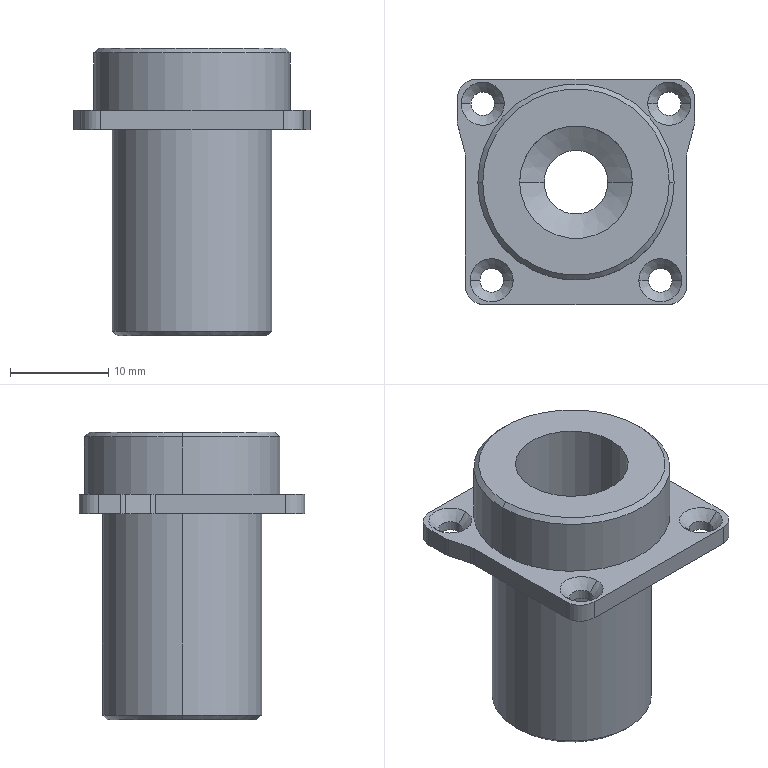NC program | NX | posted with a generic post | part box 24.2 x 23 x 29.342 mm
Whole program:
N10 G17 G21 G94 G90
(PLANAR_MILL , TOOL : D50面刀)
N12 T01 M6
N14 G53
N16 G17 G0 G90 X-0.5 Y-40.1 S4500 M3
N18 G43 Z20. H1
N20 Z2.
N22 G94 G1 Z0. F600.
N24 Y-12.1
N26 Y12.1
N28 Y40.1
N30 Z2.
N32 G0 Z20.
N34 M5
(动态粗 , TOOL : D8-25-D8-60-3T-ROUGH)
N36 T02 M6
N38 G53
N40 G17 G0 G90 X0.429 Y20.061 S6500 M3
N42 G43 Z20. H2
N44 Z-20.35
N46 G94 G1 X0.43 Y20.036 Z-20.506 F3000.
N48 X0.431 Y20.011 Z-20.568
N50 X0.432 Y19.986 Z-20.613
N52 X0.434 Y19.961 Z-20.65
N54 X0.435 Y19.936 Z-20.681
N56 X0.436 Y19.911 Z-20.707
N58 X0.437 Y19.886 Z-20.73
N60 X0.438 Y19.861 Z-20.75
N62 X0.44 Y19.836 Z-20.768
N64 X0.441 Y19.811 Z-20.783
N66 X0.442 Y19.786 Z-20.797
N68 X0.443 Y19.761 Z-20.808
N70 X0.444 Y19.736 Z-20.818
N72 X0.446 Y19.711 Z-20.827
N74 X0.447 Y19.686 Z-20.834
N76 X0.448 Y19.661 Z-20.84
N78 X0.449 Y19.636 Z-20.844
N80 X0.45 Y19.611 Z-20.847
N82 X0.452 Y19.586 Z-20.849
N84 X0.453 Y19.561 Z-20.85
N86 X0.516 Y18.254
N88 G3 X0.99 Y17.557 R0.809
N90 X3.846 Y16.911 R8.421
N92 X10.454 Y16.699 R95.671
N94 G2 X13.454 Y14.982 R4.502
N96 X15.139 Y11.177 R8.706
N98 X15.634 Y5.867 R30.68
N100 X15.682 Y-11.513 R786.797
N102 X13.805 Y-14.605 R4.562
N104 X9.896 Y-16.198 R9.151
N106 X4.22 Y-16.649 R35.622
N108 X-10.491 Y-16.683 R805.734
N110 X-13.56 Y-14.878 R4.516
N112 X-15.165 Y-11.103 R8.828
N114 X-15.645 Y-5.49 R33.344
N116 X-15.684 Y11.491 R889.228
N118 X-13.878 Y14.559 R4.516
N120 X-10.162 Y16.152 R8.771
N122 X-4.791 Y16.637 R31.617
N124 X-0.773 Y16.63 R41.473
N126 G3 X4.691 Y16.093 R140.668
N128 G2 X8.411 Y15.922 R235.686
N130 X12.726 Y13.128 R6.126
N132 X14.387 Y8.598 R11.548
N134 X14.854 Y2.08 R44.461
N136 X14.885 Y-9.139 R699.319
N138 X12.271 Y-13.604 R5.956
N140 X7.888 Y-15.33 R10.972
N142 X1.736 Y-15.839 R38.769
N144 X-8.283 Y-15.875 R261.049
N146 X-12.684 Y-13.17 R5.998
N148 X-14.357 Y-8.763 R11.22
N150 X-14.846 Y-2.489 R40.851
N152 X-14.877 Y9.271 R378.584
N154 X-12.178 Y13.678 R5.986
N156 X-7.775 Y15.354 R11.211
N158 X0.715 Y15.603 R31.798
N160 G3 X6.56 Y15.199 R403.425
N162 G2 X11.957 Y11.622 R7.16
N164 X13.598 Y6.695 R13.544
N166 X14.047 Y-0.005 R50.406
N168 X14.067 Y-7.426 R173.713
N170 X10.784 Y-12.81 R6.926
N172 X5.96 Y-14.546 R12.736
N174 X-0.496 Y-15.039 R44.911
N176 X-6.435 Y-15.064 R119.403
N178 X-11.831 Y-11.759 R6.914
N180 X-13.555 Y-6.914 R12.852
N182 X-14.048 Y-0.098 R47.277
N184 X-14.066 Y7.461 R161.04
N186 X-10.706 Y12.864 R6.932
N188 X-5.751 Y14.58 R12.98
N190 X0.415 Y14.758 R29.731
N192 X5.144 Y14.453 R98.986
N194 X11.196 Y10.249 R7.942
N196 X12.796 Y5.122 R15.097
N198 X13.082 Y2.379 R49.141
N200 G1 X13.293 Y0.888
N202 G2 X13.259 Y-5.834 R187.6
N204 X9.361 Y-12.067 R7.65
N206 X4.26 Y-13.762 R14.309
N208 X-2.558 Y-14.242 R51.282
N210 X-5.85 Y-14.118 R16.984
N212 X-11.092 Y-10.317 R7.64
N214 X-12.771 Y-5.208 R14.441
N216 X-13.25 Y1.911 R53.484
N218 X-13.225 Y6.169 R46.387
N220 X-9.465 Y12.006 R7.59
N222 X-3.951 Y13.739 R13.317
N224 X4.014 Y13.658 R40.114
N226 X10.324 Y9.169 R8.456
N228 X11.402 Y6.559 R14.95
N230 G1 X11.928 Y5.7
N232 X12.601 Y4.163
N234 G2 X13.084 Y2.371 R18.917
N236 G1 X13.293 Y0.888
N238 X13.3 Y-0.789
N240 X13.079 Y-2.452
N242 G3 X12.63 Y-4.819 R16.341
N244 G2 X7.704 Y-11.516 R8.73
N246 X2.295 Y-13.038 R16.937
N248 X-3.689 Y-13.355 R35.26
N250 X-10.12 Y-9.354 R8.001
N252 X-11.891 Y-4.223 R14.57
N254 X-12.436 Y3.19 R50.486
N256 X-11.797 Y7.249 R9.919
N258 X-7.419 Y11.614 R8.469
N260 X-1.95 Y12.889 R15.636
N262 X3.019 Y12.805 R23.293
N264 X8.22 Y9.955 R8.579
N266 G1 X8.764 Y9.572
N268 X9.992 Y8.429
N270 X11.053 Y7.131
N272 X11.428 Y6.516
N274 X11.053 Y7.131
N276 X9.992 Y8.429
N278 X8.764 Y9.572
N280 X7.392 Y10.538
N282 G3 X5.512 Y11.463 R17.868
N284 X0.467 Y12.382 R14.195
N286 X-5.693 Y11.598 R18.155
N288 X-10.208 Y8.351 R8.688
N290 X-11.688 Y3.96 R9.487
N292 X-11.08 Y-5.339 R29.025
N294 X-8.797 Y-9.934 R10.858
N296 X-3.703 Y-12.54 R8.228
N298 X5.606 Y-11.71 R21.642
N300 X10.229 Y-8.511 R9.469
N302 X11.104 Y-7.056 R10.021
N304 G1 X11.964 Y-5.629
N306 X12.63 Y-4.079
N308 X12.949 Y-2.922
N310 X12.63 Y-4.079
N312 X11.964 Y-5.629
N314 X11.093 Y-7.074
N316 X10.032 Y-8.386
N318 X8.801 Y-9.542
N320 X7.425 Y-10.518
N322 X5.928 Y-11.297
N324 X4.339 Y-11.864
N326 X2.687 Y-12.209
N328 X1.003 Y-12.325
N330 G2 X-2.002 Y-11.954 R14.341
N332 X-6.309 Y-10.392 R9.852
N334 X-9.345 Y-6.682 R9.353
N336 X-10.208 Y-5.126 R17.403
N338 G1 X-10.784 Y-3.612
N340 X-11.156 Y-2.035
N342 X-11.318 Y-0.423
N344 X-11.267 Y1.197
N346 G2 X-10.661 Y4.561 R41.802
N348 X-6.023 Y10.097 R8.435
N350 G1 X-5.47 Y10.49
N352 X-3.962 Y11.282
N354 X-2.36 Y11.858
N356 X-0.693 Y12.208
N358 X1.004 Y12.325
N360 X2.679 Y12.21
N362 X1.004 Y12.325
N364 X-0.693 Y12.208
N366 X-2.36 Y11.858
N368 X-3.962 Y11.282
N370 X-5.47 Y10.49
N372 X-6.79 Y9.551
N374 X-7.976 Y8.446
N376 X-9.006 Y7.196
N378 X-9.864 Y5.821
N380 X-10.533 Y4.346
N382 X-11.004 Y2.796
N384 X-11.267 Y1.197
N386 X-11.318 Y-0.423
N388 X-11.156 Y-2.035
N390 X-10.784 Y-3.612
N392 X-10.208 Y-5.126
N394 G3 X-9.345 Y-6.682 R17.403
N396 G1 X-8.489 Y-7.865
N398 X-7.376 Y-9.042
N400 X-6.117 Y-10.062
N402 G3 X-2.002 Y-11.954 R13.361
N404 G2 X-1.458 Y-12.57 R0.802
N406 G1 X-1.14 Y-14.109 Z-20.75
N408 X-1.099 Y-14.308 F15000.
N410 X-1.048 Y-14.504
N412 G3 X-0.234 Y-15.016 R0.8
N414 G1 X0.903 Y-14.921
N416 X2.038 Y-14.79
N418 G3 X4.321 Y-14.371 R24.733
N420 X6.908 Y-13.481 R14.428
N422 X8.603 Y-12.513 R11.909
N424 G1 X10.346 Y-11.305
N426 G3 X11.628 Y-10.293 R18.424
N428 X12.658 Y-9.047 R5.858
N430 X14.327 Y-6.159 R39.578
N432 X15.172 Y-4.349 R23.342
N434 X15.743 Y-0.988 R8.479
N436 G1 X15.709 Y0.018
N438 X15.664 Y1.025
N440 G3 X14.752 Y5.24 R15.147
N442 G1 X14.258 Y6.543
N444 G3 X12.967 Y8.697 R9.153
N446 X10.921 Y10.825 R16.919
N448 G1 X9.318 Y12.223
N450 G3 X8.424 Y12.331 R0.801
N452 G1 X8.332 Y12.283
N454 X6.937 Y11.559 Z-20.85 F3000.
N456 X6.681 Y11.423
N458 X6.417 Y11.301
N460 G2 X5.902 Y11.308 R0.808
N462 G1 X4.321 Y11.869
N464 X2.853 Y12.174
N466 G2 X2.212 Y12.895 R0.808
N468 G1 X2.097 Y14.219
N470 X2.095 Y14.244 Z-20.849
N472 X2.093 Y14.269 Z-20.847
N474 X2.091 Y14.294 Z-20.844
N476 X2.089 Y14.319 Z-20.84
N478 X2.086 Y14.344 Z-20.834
N480 X2.084 Y14.369 Z-20.827
N482 X2.082 Y14.394 Z-20.818
N484 X2.08 Y14.419 Z-20.808
N486 X2.078 Y14.443 Z-20.797
N488 X2.076 Y14.468 Z-20.783
N490 X2.073 Y14.493 Z-20.768
N492 X2.071 Y14.518 Z-20.75
N494 X2.069 Y14.543 Z-20.73
N496 X2.067 Y14.568 Z-20.707
N498 X2.065 Y14.593 Z-20.681
N500 X2.063 Y14.618 Z-20.65
N502 X2.06 Y14.643 Z-20.613
N504 X2.058 Y14.668 Z-20.568
N506 X2.056 Y14.692 Z-20.506
N508 X2.054 Y14.717 Z-20.35
N510 G0 Z20.
N512 M5
(DRILLING , TOOL : 倒角D4-90度)
N514 T05 M6
N516 G53
N518 G17 G0 G90 X1. Y0. S2000 M3
N520 G43 Z20. H5
N522 G94 G81 G99 Z-1. F200. R3.
N524 G80
N526 G0 X1. Y0. Z20.
N528 M5
(DRILLING_COPY , TOOL : 钻头D6.5-73-105)
N530 T06 M6
N532 G53
N534 G17 G0 G90 X1. Y0. S2000 M3
N536 G43 Z20. H6
N538 G94 G83 G99 Z-32. F200. Q2. R3.
N540 G80
N542 G0 X1. Y0. Z20.
N544 M5
(动态粗_1 , TOOL : D4-12-D4-50-3T-ROUGH)
N546 T04 M6
N548 G53
N550 G17 G0 G90 X1. Y0. S5500 M3
N552 G43 Z20. H4
N554 Z-9.25
N556 G94 G1 Z-9.75 F1500.
N558 G3 X0.983 Y-0.392 R0.198
N560 X1.196 Y0.415 R0.42
N562 X1.105 Y-0.473 R-0.467
N564 X0.551 Y0.282 R-0.514
N566 X1.453 Y0.402 R-0.565
N568 X1.019 Y-0.64 R-0.618
N570 X0.554 Y0.544 R-0.677
N572 X1.783 Y0.083 R-0.74
N574 X0.511 Y-0.666 R-0.806
N576 X1.06 Y0.919 R-0.877
N578 X1.529 Y-0.837 R-0.95
N580 X-0.003 Y0.334 R-1.028
N582 X2.106 Y0.383 R-1.111
N584 X0.222 Y-0.946 R-1.197
N586 X1.375 Y1.287 R-1.285
N588 X1.252 Y-1.395 R-1.376
N590 X0.226 Y1.305 R-1.47
N592 X2.331 Y-0.933 R-1.568
N594 X-0.651 Y0.439 R-1.669
N596 X2.829 Y0.208 R-1.773
N598 X-0.732 Y-0.822 R-1.88
N600 X2.557 Y1.349 R-1.989
N602 X-0.217 Y-1.762 R-2.1
N604 X1.893 Y2.1 R-2.212
N606 X0.518 Y-2.325 R-2.327
N608 X1.127 Y2.508 R-2.444
N610 X1.307 Y-2.6 R-2.563
N612 X0.246 Y2.644 R-2.685
N614 X2.252 Y-2.583 R-2.809
N616 X-0.664 Y2.491 R-2.934
N618 X3.08 Y-2.338 R-3.062
N620 X-1.336 Y2.257 R-3.19
N622 X3.611 Y-2.163 R-3.319
N624 X-1.599 Y2.352 R3.447
N626 X3.801 Y-2.339 R-3.577
N628 X-1.848 Y2.467 R3.708
N630 X4.026 Y-2.485 R-3.841
N632 X3.583 Y3.015 R3.941
N634 X0.212 Y3.891 R4.103
N636 X-2.093 Y2.488 R4.209
N638 X-2.969 Y-0.064 R4.209
N640 X-2.018 Y-2.579 R4.208
N642 X0.318 Y-3.911 R4.208
N644 X2.965 Y-3.45 R4.203
N646 X4.585 Y1.699 R4.003
N648 X3.606 Y2.995 R4.316
N650 X2.976 Y2.868 R0.404
N652 G1 X2.747 Y2.396
N654 X2.736 Y2.374 Z-9.749
N656 X2.725 Y2.351 Z-9.747
N658 X2.714 Y2.329 Z-9.744
N660 X2.704 Y2.306 Z-9.74
N662 X2.693 Y2.284 Z-9.734
N664 X2.682 Y2.261 Z-9.727
N666 X2.671 Y2.239 Z-9.718
N668 X2.66 Y2.216 Z-9.708
N670 X2.649 Y2.194 Z-9.697
N672 X2.638 Y2.171 Z-9.683
N674 X2.627 Y2.149 Z-9.668
N676 X2.616 Y2.126 Z-9.65
N678 X2.605 Y2.104 Z-9.63
N680 X2.594 Y2.081 Z-9.607
N682 X2.583 Y2.059 Z-9.581
N684 X2.573 Y2.036 Z-9.55
N686 X2.562 Y2.014 Z-9.513
N688 X2.551 Y1.991 Z-9.468
N690 X2.54 Y1.969 Z-9.406
N692 X2.529 Y1.946 Z-9.25
N694 G0 Z20.
(动态粗_1_COPY , TOOL : D4-12-D4-50-3T-ROUGH)
N696 X1. Y0.
N698 Z-15.6
N700 G3 X0.617 Y0.017 R0.195
N702 X1.304 Y-0.392 R0.418
N704 X0.486 Y0.065 R-0.504
N706 X1.618 Y-0.089 R-0.572
N708 X0.334 Y0.002 R-0.644
N710 X1.775 Y0.051 R-0.723
N712 X0.174 Y-0.19 R-0.81
N714 X1.922 Y0.272 R-0.905
N716 X0.056 Y-0.479 R-1.008
N718 X2.006 Y0.611 R-1.119
N720 X-0.04 Y-0.78 R-1.237
N722 X2.141 Y0.85 R-1.361
N724 X-0.118 Y-1.099 R-1.494
N726 X2.297 Y1.094 R1.632
N728 X0.439 Y-1.715 R-1.752
N730 X-0.797 Y-0.106 R-1.799
N732 X-0.289 Y-0.436 R0.404
N734 G1 X0.231 Y-0.292
N736 X0.255 Y-0.285 Z-15.599
N738 X0.279 Y-0.278 Z-15.597
N740 X0.303 Y-0.272 Z-15.594
N742 X0.327 Y-0.265 Z-15.59
N744 X0.351 Y-0.258 Z-15.584
N746 X0.376 Y-0.252 Z-15.577
N748 X0.4 Y-0.245 Z-15.568
N750 X0.424 Y-0.238 Z-15.558
N752 X0.448 Y-0.232 Z-15.547
N754 X0.472 Y-0.225 Z-15.533
N756 X0.496 Y-0.218 Z-15.518
N758 X0.52 Y-0.212 Z-15.5
N760 X0.544 Y-0.205 Z-15.48
N762 X0.568 Y-0.198 Z-15.457
N764 X0.592 Y-0.192 Z-15.431
N766 X0.617 Y-0.185 Z-15.4
N768 X0.641 Y-0.178 Z-15.363
N770 X0.665 Y-0.172 Z-15.318
N772 X0.689 Y-0.165 Z-15.256
N774 X0.713 Y-0.158 Z-15.1
N776 G0 Z20.
N778 X0.917 Y-0.493
N780 Z-14.625
N782 G1 X0.921 Y-0.468 Z-14.781
N784 X0.925 Y-0.444 Z-14.843
N786 X0.93 Y-0.419 Z-14.888
N788 X0.934 Y-0.394 Z-14.925
N790 X0.938 Y-0.37 Z-14.956
N792 X0.942 Y-0.345 Z-14.982
N794 X0.946 Y-0.321 Z-15.005
N796 X0.95 Y-0.296 Z-15.025
N798 X0.954 Y-0.271 Z-15.043
N800 X0.959 Y-0.247 Z-15.058
N802 X0.963 Y-0.222 Z-15.072
N804 X0.967 Y-0.197 Z-15.083
N806 X0.971 Y-0.173 Z-15.093
N808 X0.975 Y-0.148 Z-15.102
N810 X0.979 Y-0.123 Z-15.109
N812 X0.983 Y-0.099 Z-15.115
N814 X0.988 Y-0.074 Z-15.119
N816 X0.992 Y-0.049 Z-15.122
N818 X0.996 Y-0.025 Z-15.124
N820 X1. Y0. Z-15.125
N822 X1.219 Y1.306
N824 G3 X1.015 Y1.727 R0.405
N826 X0.624 Y1.801 R0.568
N828 X2.756 Y-0.565 R-1.84
N830 X0.609 Y1.796 R1.846
N832 X0.37 Y1.246 R0.404
N834 G1 X0.591 Y0.757
N836 X0.601 Y0.734 Z-15.124
N838 X0.612 Y0.712 Z-15.122
N840 X0.622 Y0.689 Z-15.119
N842 X0.632 Y0.666 Z-15.115
N844 X0.643 Y0.643 Z-15.109
N846 X0.653 Y0.621 Z-15.102
N848 X0.663 Y0.598 Z-15.093
N850 X0.673 Y0.575 Z-15.083
N852 X0.684 Y0.552 Z-15.072
N854 X0.694 Y0.529 Z-15.058
N856 X0.704 Y0.507 Z-15.043
N858 X0.715 Y0.484 Z-15.025
N860 X0.725 Y0.461 Z-15.005
N862 X0.735 Y0.438 Z-14.982
N864 X0.746 Y0.416 Z-14.956
N866 X0.756 Y0.393 Z-14.925
N868 X0.766 Y0.37 Z-14.888
N870 X0.776 Y0.347 Z-14.843
N872 X0.787 Y0.324 Z-14.781
N874 X0.797 Y0.302 Z-14.625
N876 G0 Z20.
N878 X0.944 Y-0.497
N880 Z-14.15
N882 G1 X0.947 Y-0.472 Z-14.306
N884 X0.95 Y-0.447 Z-14.368
N886 X0.953 Y-0.422 Z-14.413
N888 X0.956 Y-0.398 Z-14.45
N890 X0.958 Y-0.373 Z-14.481
N892 X0.961 Y-0.348 Z-14.507
N894 X0.964 Y-0.323 Z-14.53
N896 X0.967 Y-0.298 Z-14.55
N898 X0.969 Y-0.273 Z-14.568
N900 X0.972 Y-0.248 Z-14.583
N902 X0.975 Y-0.224 Z-14.597
N904 X0.978 Y-0.199 Z-14.608
N906 X0.981 Y-0.174 Z-14.618
N908 X0.983 Y-0.149 Z-14.627
N910 X0.986 Y-0.124 Z-14.634
N912 X0.989 Y-0.099 Z-14.64
N914 X0.992 Y-0.075 Z-14.644
N916 X0.994 Y-0.05 Z-14.647
N918 X0.997 Y-0.025 Z-14.649
N920 X1. Y0. Z-14.65
N922 X1.155 Y1.387
N924 G3 X0.887 Y1.814 R0.405
N926 X0.602 Y1.844 R0.963
N928 X-0.398 Y-1.267 R1.896
N930 X2.75 Y0.704 R1.889
N932 X0.617 Y1.847 R1.922
N934 X0.357 Y1.266 R0.404
N936 G1 X0.599 Y0.808
N938 X0.61 Y0.786 Z-14.649
N940 X0.622 Y0.764 Z-14.647
N942 X0.634 Y0.741 Z-14.644
N944 X0.645 Y0.719 Z-14.64
N946 X0.657 Y0.697 Z-14.634
N948 X0.669 Y0.675 Z-14.627
N950 X0.68 Y0.653 Z-14.618
N952 X0.692 Y0.631 Z-14.608
N954 X0.704 Y0.609 Z-14.597
N956 X0.715 Y0.587 Z-14.583
N958 X0.727 Y0.565 Z-14.568
N960 X0.739 Y0.542 Z-14.55
N962 X0.75 Y0.52 Z-14.53
N964 X0.762 Y0.498 Z-14.507
N966 X0.774 Y0.476 Z-14.481
N968 X0.785 Y0.454 Z-14.45
N970 X0.797 Y0.432 Z-14.413
N972 X0.809 Y0.41 Z-14.368
N974 X0.82 Y0.388 Z-14.306
N976 X0.832 Y0.366 Z-14.15
N978 G0 Z20.
N980 X1.497 Y-0.058
N982 Z-13.675
N984 G1 X1.472 Y-0.055 Z-13.831
N986 X1.447 Y-0.052 Z-13.893
N988 X1.422 Y-0.049 Z-13.938
N990 X1.397 Y-0.046 Z-13.975
N992 X1.372 Y-0.043 Z-14.006
N994 X1.348 Y-0.04 Z-14.032
N996 X1.323 Y-0.038 Z-14.055
N998 X1.298 Y-0.035 Z-14.075
N1000 X1.273 Y-0.032 Z-14.093
N1002 X1.248 Y-0.029 Z-14.108
N1004 X1.223 Y-0.026 Z-14.122
N1006 X1.199 Y-0.023 Z-14.133
N1008 X1.174 Y-0.02 Z-14.143
N1010 X1.149 Y-0.017 Z-14.152
N1012 X1.124 Y-0.014 Z-14.159
N1014 X1.099 Y-0.012 Z-14.165
N1016 X1.074 Y-0.009 Z-14.169
N1018 X1.05 Y-0.006 Z-14.172
N1020 X1.025 Y-0.003 Z-14.174
N1022 X1. Y0. Z-14.175
N1024 X-0.418 Y0.165
N1026 G3 X-0.86 Y-0.154 R0.404
N1028 X-0.783 Y-0.72 R1.015
N1030 X2.93 Y0.006 R1.93
N1032 X1.878 Y1.711 R2.034
N1034 X-0.922 Y-0.068 R1.936
N1036 G1 X-0.876 Y-0.334
N1038 G3 X-0.286 Y-0.621 R0.404
N1040 G1 X0.148 Y-0.387
N1042 X0.17 Y-0.376 Z-14.174
N1044 X0.192 Y-0.364 Z-14.172
N1046 X0.214 Y-0.352 Z-14.169
N1048 X0.236 Y-0.34 Z-14.165
N1050 X0.258 Y-0.328 Z-14.159
N1052 X0.28 Y-0.316 Z-14.152
N1054 X0.302 Y-0.304 Z-14.143
N1056 X0.324 Y-0.293 Z-14.133
N1058 X0.346 Y-0.281 Z-14.122
N1060 X0.368 Y-0.269 Z-14.108
N1062 X0.39 Y-0.257 Z-14.093
N1064 X0.412 Y-0.245 Z-14.075
N1066 X0.434 Y-0.233 Z-14.055
N1068 X0.456 Y-0.221 Z-14.032
N1070 X0.478 Y-0.21 Z-14.006
N1072 X0.5 Y-0.198 Z-13.975
N1074 X0.522 Y-0.186 Z-13.938
N1076 X0.544 Y-0.174 Z-13.893
N1078 X0.566 Y-0.162 Z-13.831
N1080 X0.588 Y-0.15 Z-13.675
N1082 G0 Z20.
N1084 X1.496 Y-0.067
N1086 Z-12.25
N1088 G1 X1.471 Y-0.063 Z-12.406
N1090 X1.446 Y-0.06 Z-12.468
N1092 X1.421 Y-0.057 Z-12.513
N1094 X1.396 Y-0.053 Z-12.55
N1096 X1.372 Y-0.05 Z-12.581
N1098 X1.347 Y-0.047 Z-12.607
N1100 X1.322 Y-0.043 Z-12.63
N1102 X1.297 Y-0.04 Z-12.65
N1104 X1.273 Y-0.037 Z-12.668
N1106 X1.248 Y-0.033 Z-12.683
N1108 X1.223 Y-0.03 Z-12.697
N1110 X1.198 Y-0.027 Z-12.708
N1112 X1.173 Y-0.023 Z-12.718
N1114 X1.149 Y-0.02 Z-12.727
N1116 X1.124 Y-0.017 Z-12.734
N1118 X1.099 Y-0.013 Z-12.74
N1120 X1.074 Y-0.01 Z-12.744
N1122 X1.05 Y-0.007 Z-12.747
N1124 X1.025 Y-0.003 Z-12.749
N1126 X1. Y0. Z-12.75
N1128 X-0.478 Y0.199
N1130 G3 X-0.882 Y0.001 R0.405
N1132 X-0.77 Y-1.26 R1.243
N1134 X3.239 Y-0.108 R2.192
N1136 X-1.154 Y0.657 R2.25
N1138 X-1.246 Y-0.732 R1.877
N1140 X0.572 Y2.323 R-2.358
N1142 X-1.341 Y-0.21 R2.359
N1144 X-0.807 Y-0.532 R0.404
N1146 G1 X-0.33 Y-0.363
N1148 X-0.306 Y-0.355 Z-12.749
N1150 X-0.283 Y-0.347 Z-12.747
N1152 X-0.259 Y-0.338 Z-12.744
N1154 X-0.236 Y-0.33 Z-12.74
N1156 X-0.212 Y-0.322 Z-12.734
N1158 X-0.188 Y-0.313 Z-12.727
N1160 X-0.165 Y-0.305 Z-12.718
N1162 X-0.141 Y-0.297 Z-12.708
N1164 X-0.118 Y-0.288 Z-12.697
N1166 X-0.094 Y-0.28 Z-12.683
N1168 X-0.071 Y-0.272 Z-12.668
N1170 X-0.047 Y-0.263 Z-12.65
N1172 X-0.023 Y-0.255 Z-12.63
N1174 X0. Y-0.247 Z-12.607
N1176 X0.024 Y-0.238 Z-12.581
N1178 X0.047 Y-0.23 Z-12.55
N1180 X0.071 Y-0.222 Z-12.513
N1182 X0.095 Y-0.213 Z-12.468
N1184 X0.118 Y-0.205 Z-12.406
N1186 X0.142 Y-0.197 Z-12.25
N1188 G0 Z20.
N1190 X0.937 Y-0.496
N1192 Z-11.775
N1194 G1 X0.94 Y-0.471 Z-11.931
N1196 X0.943 Y-0.446 Z-11.993
N1198 X0.946 Y-0.422 Z-12.038
N1200 X0.949 Y-0.397 Z-12.075
N1202 X0.953 Y-0.372 Z-12.106
N1204 X0.956 Y-0.347 Z-12.132
N1206 X0.959 Y-0.322 Z-12.155
N1208 X0.962 Y-0.298 Z-12.175
N1210 X0.965 Y-0.273 Z-12.193
N1212 X0.968 Y-0.248 Z-12.208
N1214 X0.972 Y-0.223 Z-12.222
N1216 X0.975 Y-0.198 Z-12.233
N1218 X0.978 Y-0.174 Z-12.243
N1220 X0.981 Y-0.149 Z-12.252
N1222 X0.984 Y-0.124 Z-12.259
N1224 X0.987 Y-0.099 Z-12.265
N1226 X0.991 Y-0.074 Z-12.269
N1228 X0.994 Y-0.05 Z-12.272
N1230 X0.997 Y-0.025 Z-12.274
N1232 X1. Y0. Z-12.275
N1234 X1.244 Y1.912
N1236 G3 X1.015 Y2.328 R0.405
N1238 X-0.472 Y2.196 R1.509
N1240 X0.56 Y-2.665 R2.653
N1242 X1.746 Y2.611 R2.709
N1244 X-2.03 Y0.443 R2.73
N1246 X2.439 Y2.727 R-3.071
N1248 X-1.997 Y1.643 R3.166
N1250 X-2.418 Y-0.071 R3.839
N1252 X-0.788 Y-2.914 R3.527
N1254 X1.677 Y-3.351 R3.596
N1256 X4.089 Y-1.466 R3.544
N1258 X2.637 Y3.001 R3.447
N1260 X0.915 Y3.417 R3.846
N1262 X-1.472 Y2.361 R3.623
N1264 X-2.302 Y0.88 R3.801
N1266 X-1.91 Y0.373 R0.404
N1268 G1 X-1.386 Y0.375
N1270 X-1.361 Z-12.274
N1272 X-1.336 Z-12.272
N1274 X-1.311 Y0.376 Z-12.269
N1276 X-1.286 Z-12.265
N1278 X-1.261 Z-12.259
N1280 X-1.236 Z-12.252
N1282 X-1.211 Z-12.243
N1284 X-1.186 Z-12.233
N1286 X-1.161 Z-12.222
N1288 X-1.136 Z-12.208
N1290 X-1.111 Z-12.193
N1292 X-1.086 Y0.377 Z-12.175
N1294 X-1.061 Z-12.155
N1296 X-1.036 Z-12.132
N1298 X-1.011 Z-12.106
N1300 X-0.986 Z-12.075
N1302 X-0.961 Z-12.038
N1304 X-0.936 Z-11.993
N1306 X-0.911 Z-11.931
N1308 X-0.886 Z-11.775
N1310 G0 Z20.
N1312 M5
(PLANAR_MILL_1 , TOOL : D8-25-D8-60-3T-FINISH)
N1314 T03 M6
N1316 G53
N1318 G17 G0 G90 X2.913 Y-17.867 S4500 M3
N1320 G43 Z20. H3
N1322 Z-19.
N1324 G94 G1 Z-21. F600.
N1326 G41 X3. Y-17.375 D3
N1328 G3 X1. Y-15.375 R2.
N1330 G2 X-14.375 Y0. R15.375
N1332 X1. Y-15.375 R-15.375
N1334 G3 X-1. Y-17.375 R2.
N1336 G40
N1338 G1 X-0.913 Y-17.867
N1340 X2.913 Y-14.667
N1342 G41 X3. Y-14.175
N1344 G3 X1. Y-12.175 R2.
N1346 G2 X-11.175 Y0. R12.175
N1348 X1. Y-12.175 R-12.175
N1350 G3 X-1. Y-14.175 R2.
N1352 G1 Y-17.26
N1354 G40
N1356 X-0.913 Y-17.752
N1358 Z-19.
N1360 G0 Z20.
(PLANAR_MILL_1_COPY , TOOL : D8-25-D8-60-3T-FINISH)
N1362 X2.913 Y-14.617
N1364 Z-19.
N1366 G1 Z-21.
N1368 G41 X3. Y-14.125
N1370 G3 X1. Y-12.125 R2.
N1372 G2 X-11.125 Y0. R12.125
N1374 X1. Y-12.125 R-12.125
N1376 G3 X-1. Y-14.125 R2.
N1378 G40
N1380 G1 X-0.913 Y-14.617
N1382 Z-19.
N1384 G0 Z20.
N1386 M5
(DRILLING_1 , TOOL : D7.9)
N1388 T07 M6
N1390 G53
N1392 G17 G0 G90 X1. Y0. S3500 M3
N1394 G43 Z20. H7
N1396 G94 G81 G99 Z-15.75 F600. R-12.75
N1398 G80
N1400 G0 X1. Y0. Z20.
N1402 M5
(PLANAR_MILL_7 , TOOL : D4-12-D4-50-3T-FINISH)
N1404 T08 M6
N1406 G53
N1408 G17 G0 G90 X1.718 Y-2. S5500 M3
N1410 G43 Z20. H8
N1412 Z-7.9
N1414 G94 G1 Z-9.9 F600.
N1416 X3.125
N1418 G3 X5.125 Y0. R2.
N1420 X1. Y4.125 R4.125
N1422 X5.125 Y0. R-4.125
N1424 X3.125 Y2. R2.
N1426 G1 Y-2.
N1428 G3 X5.125 Y0. R2.
N1430 X1. Y4.125 R4.125
N1432 X5.125 Y0. R-4.125
N1434 X3.125 Y2. R2.
N1436 G1 X1.718
N1438 Z-7.9
N1440 G0 Z20.
N1442 M5
(平面铣倒角 , TOOL : 倒角D4-90度)
N1444 T05 M6
N1446 G53
N1448 G17 G0 G90 X0.004 Y10.625 S6500 M3
N1450 G43 Z20. H5
N1452 Z0.5
N1454 G94 G1 Z-1.5 F1200.
N1456 G41 X0. Y10.125 D5
N1458 G3 X1. Y9.125 R1.
N1460 G2 X10.125 Y0. R9.125
N1462 X1. Y9.125 R-9.125
N1464 G3 X2. Y10.125 R1.
N1466 G40
N1468 G1 X1.996 Y10.625
N1470 Z0.5
N1472 G0 Z20.
N1474 M5
N1476 M2